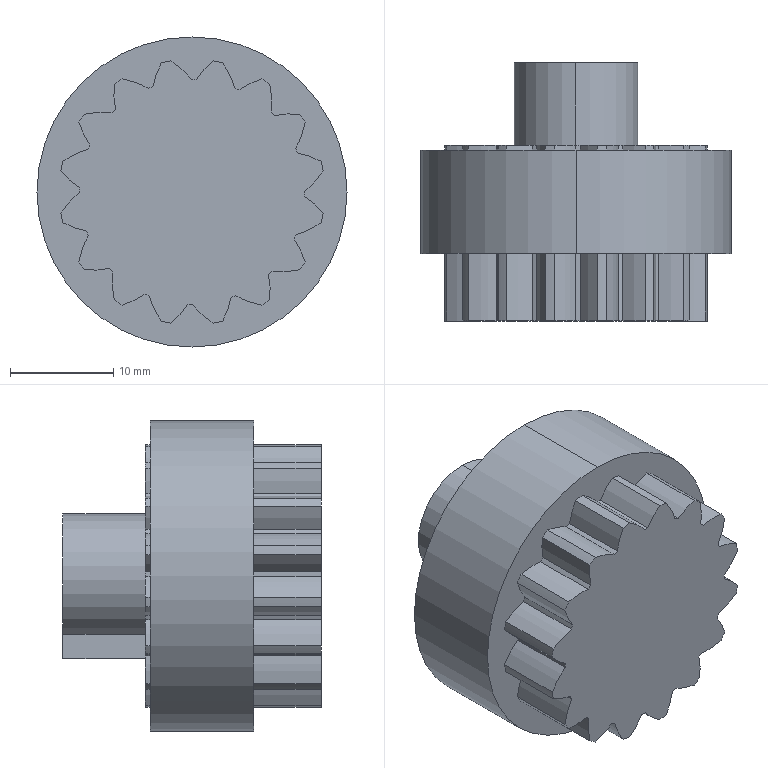Part | SolidWorks | features Cut 1, Extrusion 1, ICE 1 | 1 solid | 142 faces | box 30 x 25 x 30 mm | volume 11200 mm3 | cylinder 70 | spline 64 | plane 8 | commonest cylinder face diameters 21.75 x34 25.7 x32 12 x2 30 x2